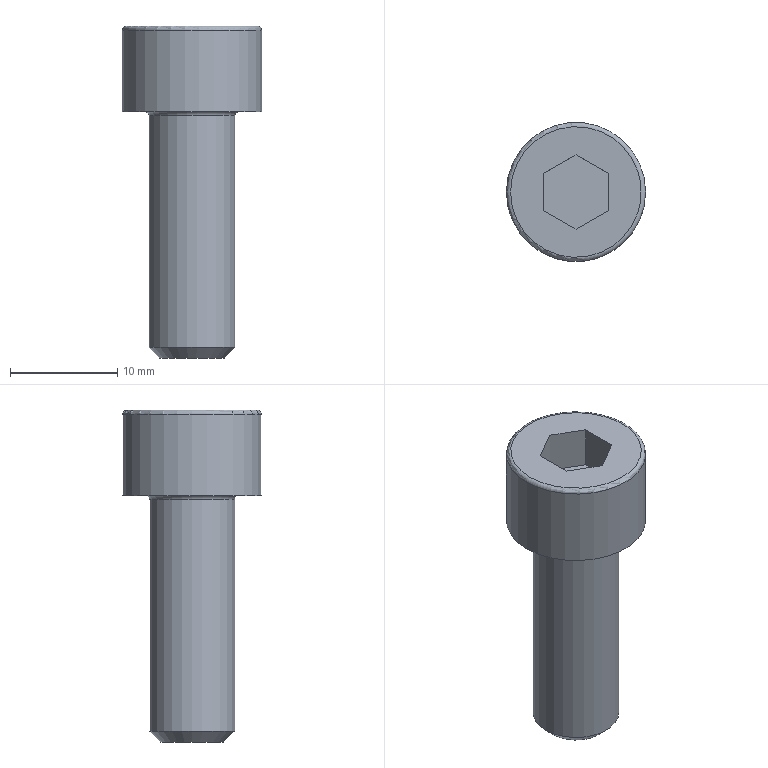Part | STEP file | solid 163 | 1 solid | 15 faces | box 13 x 13 x 31 mm | volume 2081 mm3 | plane 10 | cylinder 2 | torus 2 | cone 1 | commonest cylinder face diameters 8 x1 13 x1